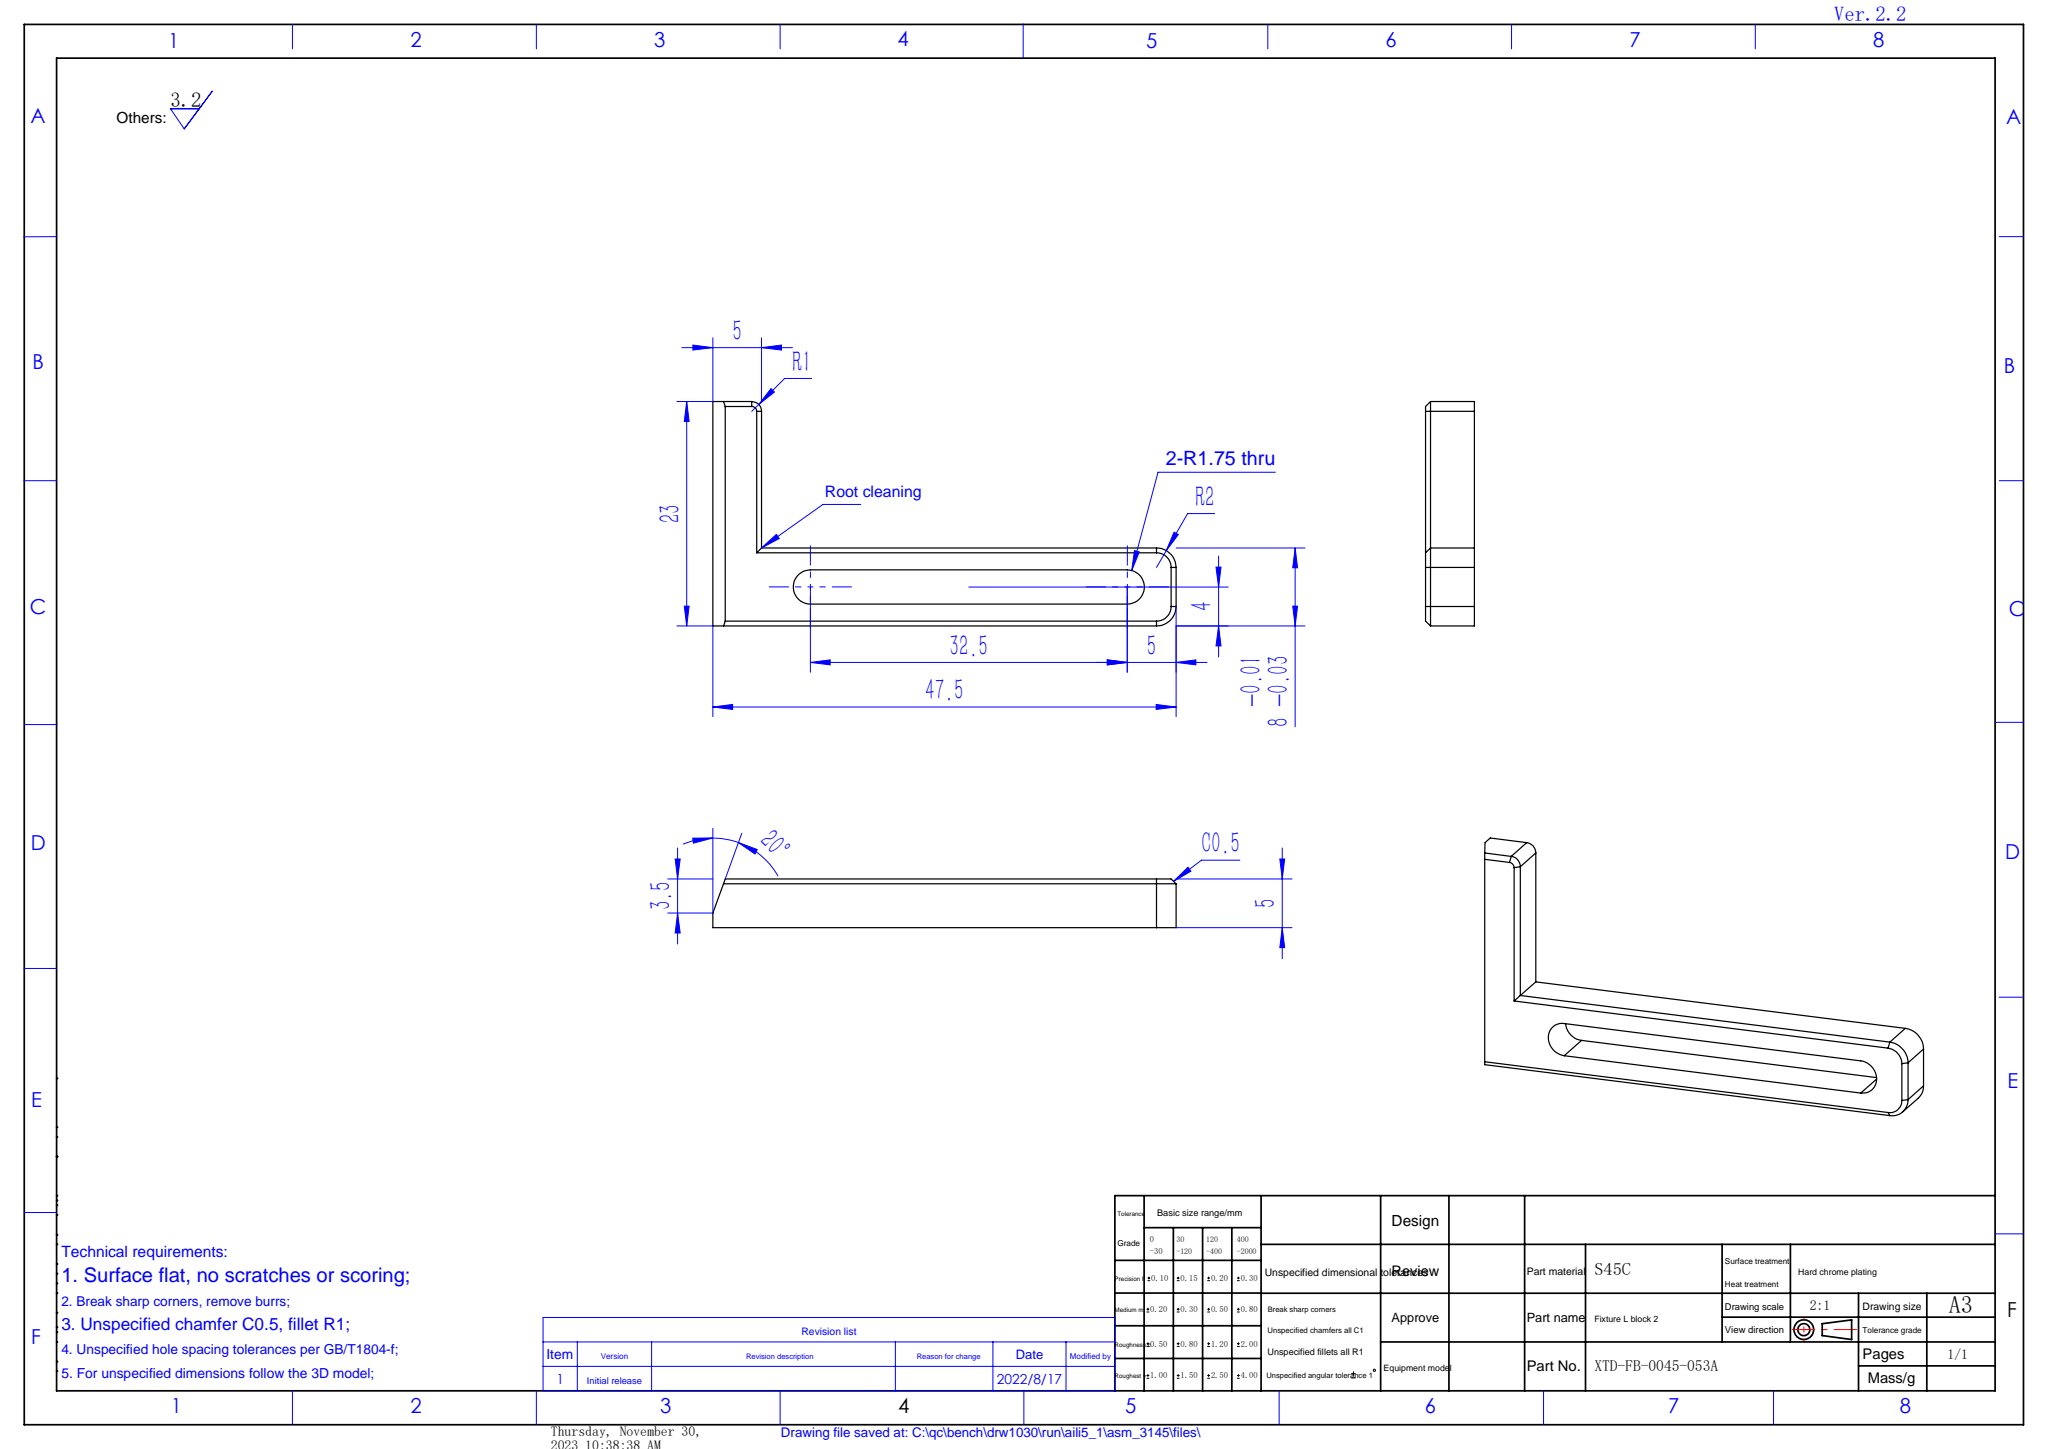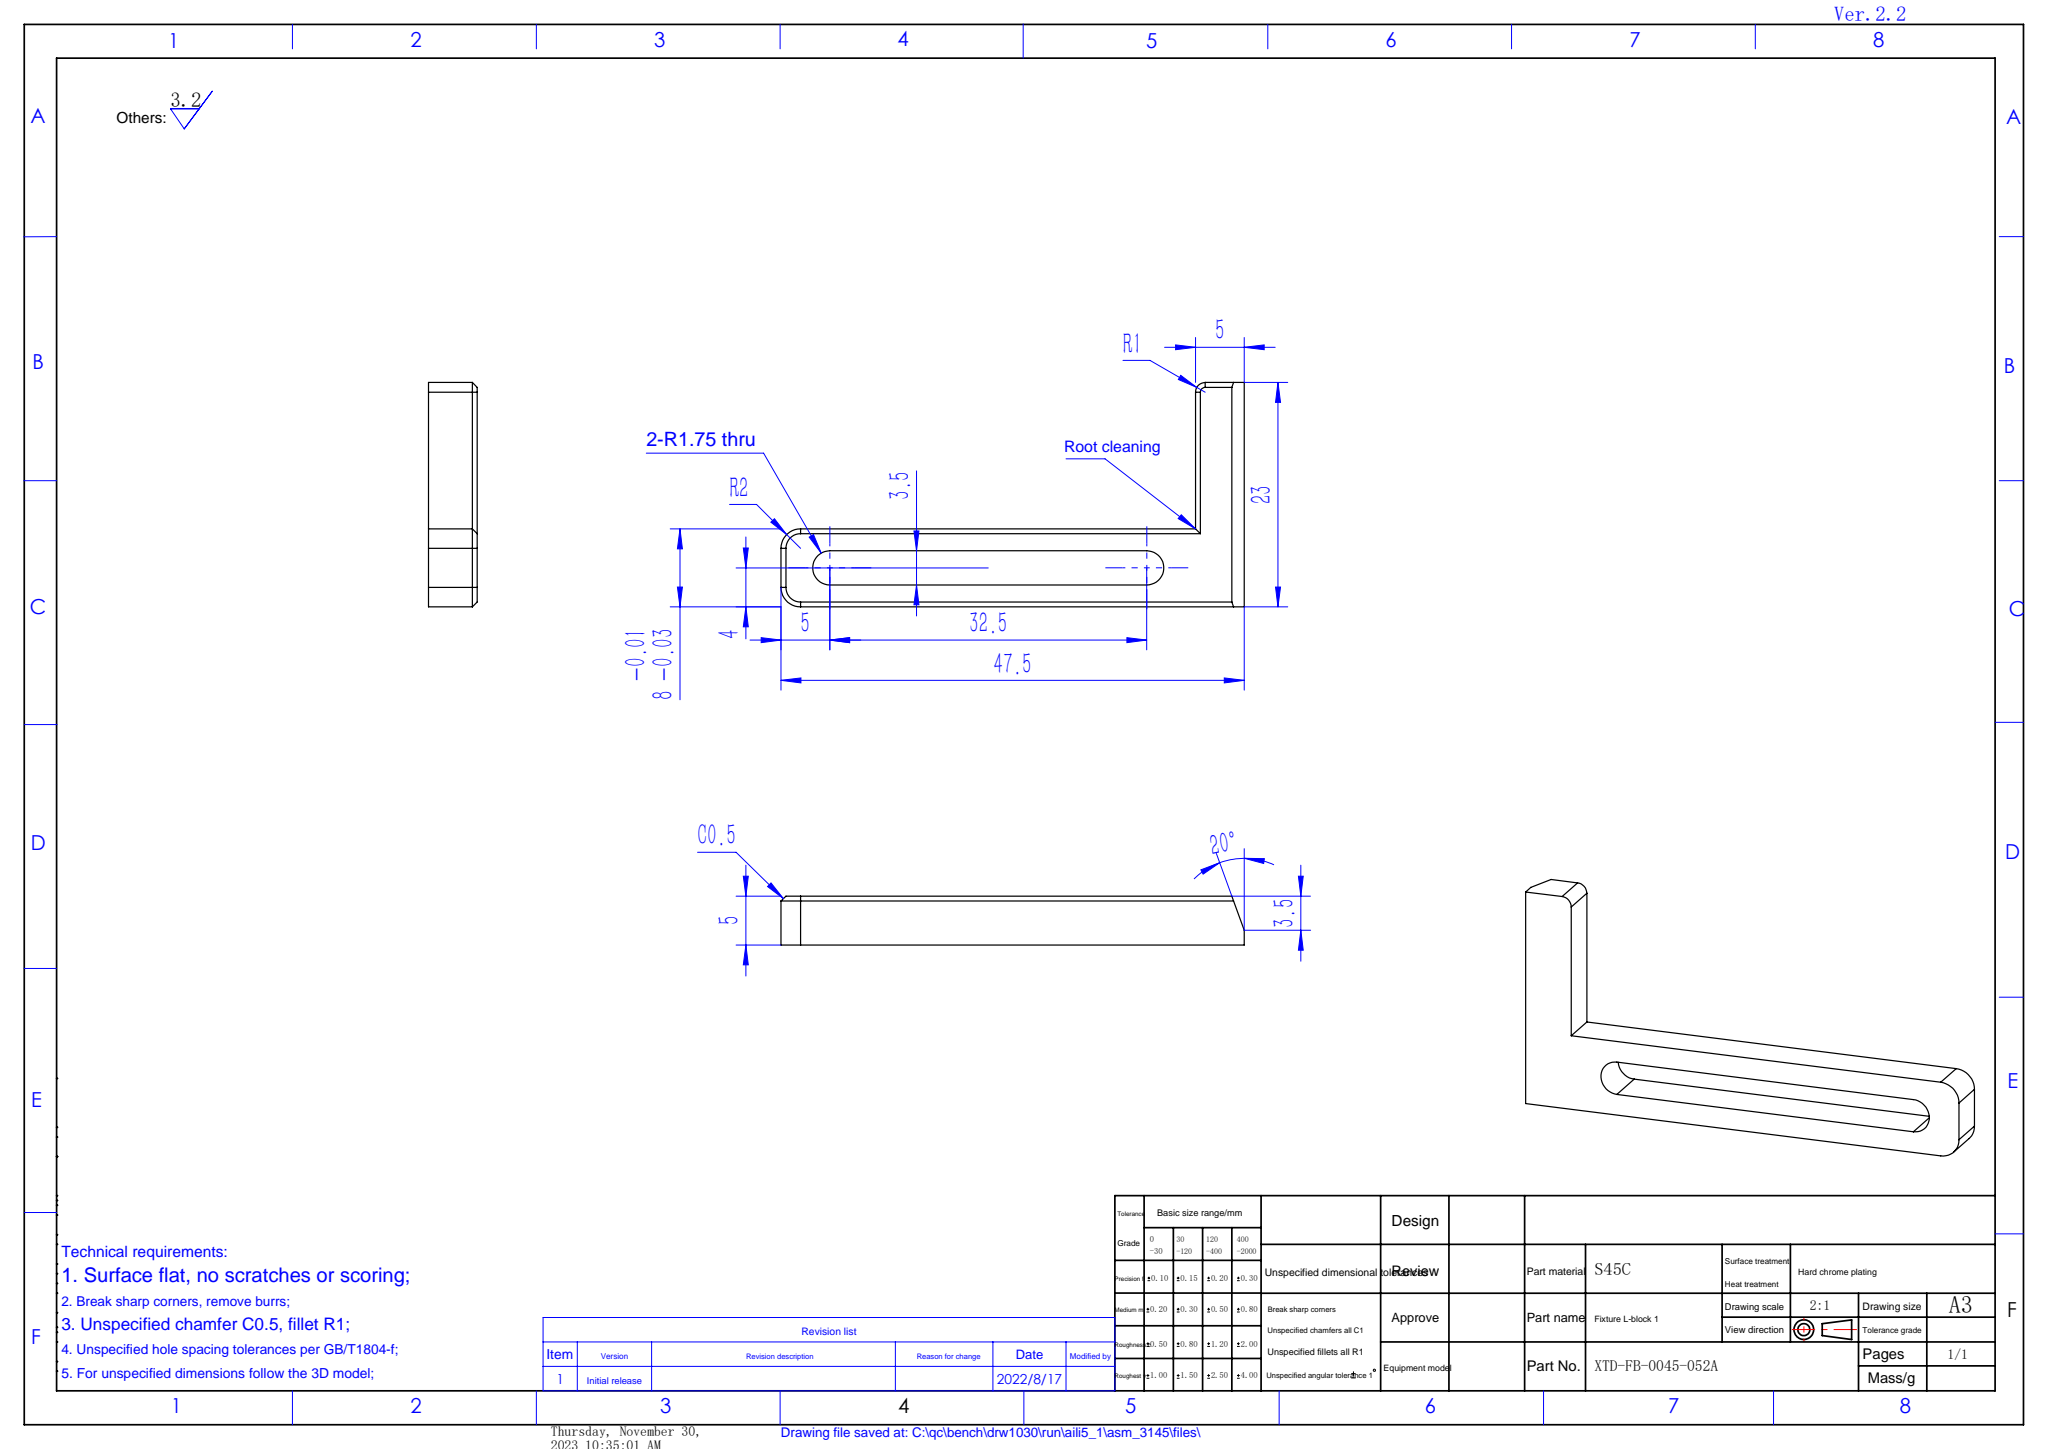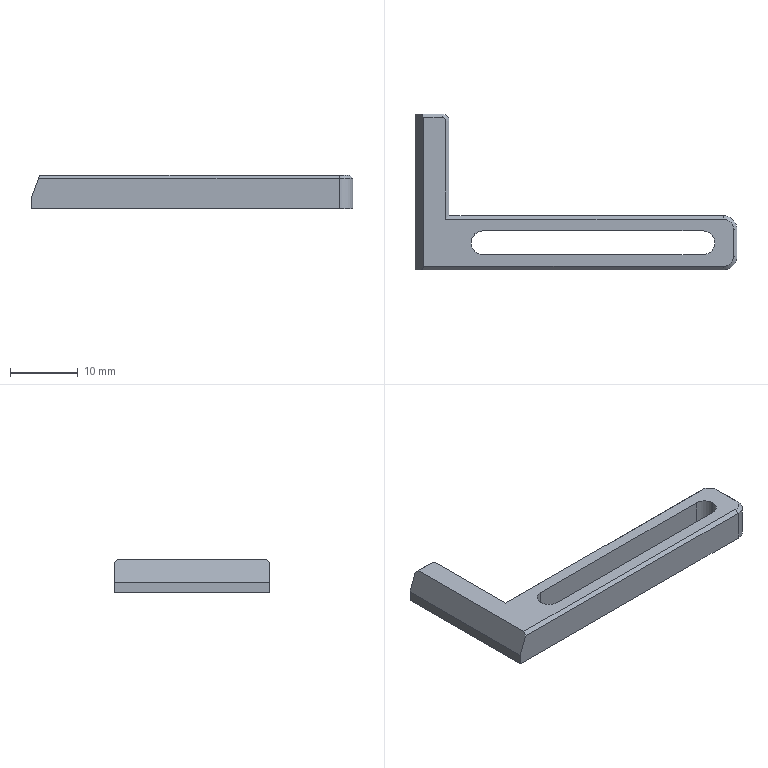Part | SolidWorks | features Fillet 2, Chamfer 1, Extrusion 1, HoleWzd 1, ICE 1 | 1 solid | 25 faces | box 47.5 x 23 x 5 mm | volume 1583 mm3 | plane 16 | cylinder 6 | cone 3 | commonest cylinder face diameters 3.5 x3 4 x2 2 x1
STEP:
#1=CARTESIAN_POINT('',(44.25,4.,0.));
#2=VERTEX_POINT('',#1);
#3=CARTESIAN_POINT('',(42.5,5.75,0.));
#4=VERTEX_POINT('',#3);
#5=CARTESIAN_POINT('',(42.5,4.,0.));
#6=DIRECTION('',(0.,0.,1.));
#7=DIRECTION('',(1.,0.,0.));
#8=AXIS2_PLACEMENT_3D('',#5,#6,#7);
#9=CIRCLE('',#8,1.75);
#10=EDGE_CURVE('',#2,#4,#9,.T.);
#11=ORIENTED_EDGE('',*,*,#10,.F.);
#12=CARTESIAN_POINT('',(44.25,4.,5.));
#13=VERTEX_POINT('',#12);
#14=CARTESIAN_POINT('',(44.25,4.,5.));
#15=DIRECTION('',(0.,0.,1.));
#16=VECTOR('',#15,1000.);
#17=LINE('',#14,#16);
#18=EDGE_CURVE('',#2,#13,#17,.T.);
#19=ORIENTED_EDGE('',*,*,#18,.T.);
#20=CARTESIAN_POINT('',(42.5,5.75,5.));
#21=VERTEX_POINT('',#20);
#22=CARTESIAN_POINT('',(42.5,4.,5.));
#23=DIRECTION('',(0.,0.,1.));
#24=DIRECTION('',(1.,0.,0.));
#25=AXIS2_PLACEMENT_3D('',#22,#23,#24);
#26=CIRCLE('',#25,1.75);
#27=EDGE_CURVE('',#13,#21,#26,.T.);
#28=ORIENTED_EDGE('',*,*,#27,.T.);
#29=CARTESIAN_POINT('',(42.5,5.75,5.));
#30=DIRECTION('',(0.,0.,1.));
#31=VECTOR('',#30,1000.);
#32=LINE('',#29,#31);
#33=EDGE_CURVE('',#4,#21,#32,.T.);
#34=ORIENTED_EDGE('',*,*,#33,.F.);
#35=EDGE_LOOP('',(#11,#19,#28,#34));
#36=FACE_OUTER_BOUND('',#35,.T.);
#37=CARTESIAN_POINT('',(42.5,4.,5.));
#38=DIRECTION('',(0.,0.,1.));
#39=DIRECTION('',(1.,0.,0.));
#40=AXIS2_PLACEMENT_3D('',#37,#38,#39);
#41=CYLINDRICAL_SURFACE('',#40,1.75);
#42=ADVANCED_FACE('',(#36),#41,.F.);
#43=CARTESIAN_POINT('',(4.5,22.,5.));
#44=VERTEX_POINT('',#43);
#45=CARTESIAN_POINT('',(4.,22.5,5.));
#46=VERTEX_POINT('',#45);
#47=CARTESIAN_POINT('',(4.,22.,5.));
#48=DIRECTION('',(0.,0.,1.));
#49=DIRECTION('',(-1.,0.,0.));
#50=AXIS2_PLACEMENT_3D('',#47,#48,#49);
#51=CIRCLE('',#50,0.5);
#52=EDGE_CURVE('',#44,#46,#51,.T.);
#53=ORIENTED_EDGE('',*,*,#52,.T.);
#54=CARTESIAN_POINT('',(1.274,22.5,5.));
#55=VERTEX_POINT('',#54);
#56=CARTESIAN_POINT('',(0.,22.5,5.));
#57=DIRECTION('',(-1.,0.,0.));
#58=VECTOR('',#57,1000.);
#59=LINE('',#56,#58);
#60=EDGE_CURVE('',#46,#55,#59,.T.);
#61=ORIENTED_EDGE('',*,*,#60,.T.);
#62=CARTESIAN_POINT('',(1.274,0.5,5.));
#63=VERTEX_POINT('',#62);
#64=CARTESIAN_POINT('',(1.274,23.,5.));
#65=DIRECTION('',(0.,-1.,0.));
#66=VECTOR('',#65,1000.);
#67=LINE('',#64,#66);
#68=EDGE_CURVE('',#55,#63,#67,.T.);
#69=ORIENTED_EDGE('',*,*,#68,.T.);
#70=CARTESIAN_POINT('',(45.5,0.5,5.));
#71=VERTEX_POINT('',#70);
#72=CARTESIAN_POINT('',(0.,0.5,5.));
#73=DIRECTION('',(1.,0.,0.));
#74=VECTOR('',#73,1000.);
#75=LINE('',#72,#74);
#76=EDGE_CURVE('',#63,#71,#75,.T.);
#77=ORIENTED_EDGE('',*,*,#76,.T.);
#78=CARTESIAN_POINT('',(47.,2.,5.));
#79=VERTEX_POINT('',#78);
#80=CARTESIAN_POINT('',(45.5,2.,5.));
#81=DIRECTION('',(0.,0.,1.));
#82=DIRECTION('',(-1.,0.,0.));
#83=AXIS2_PLACEMENT_3D('',#80,#81,#82);
#84=CIRCLE('',#83,1.5);
#85=EDGE_CURVE('',#71,#79,#84,.T.);
#86=ORIENTED_EDGE('',*,*,#85,.T.);
#87=CARTESIAN_POINT('',(47.,6.,5.));
#88=VERTEX_POINT('',#87);
#89=CARTESIAN_POINT('',(47.,0.,5.));
#90=DIRECTION('',(0.,1.,0.));
#91=VECTOR('',#90,1000.);
#92=LINE('',#89,#91);
#93=EDGE_CURVE('',#79,#88,#92,.T.);
#94=ORIENTED_EDGE('',*,*,#93,.T.);
#95=CARTESIAN_POINT('',(45.5,7.5,5.));
#96=VERTEX_POINT('',#95);
#97=CARTESIAN_POINT('',(45.5,6.,5.));
#98=DIRECTION('',(0.,0.,1.));
#99=DIRECTION('',(-1.,0.,0.));
#100=AXIS2_PLACEMENT_3D('',#97,#98,#99);
#101=CIRCLE('',#100,1.5);
#102=EDGE_CURVE('',#88,#96,#101,.T.);
#103=ORIENTED_EDGE('',*,*,#102,.T.);
#104=CARTESIAN_POINT('',(4.5,7.5,5.));
#105=VERTEX_POINT('',#104);
#106=CARTESIAN_POINT('',(0.,7.5,5.));
#107=DIRECTION('',(-1.,0.,0.));
#108=VECTOR('',#107,1000.);
#109=LINE('',#106,#108);
#110=EDGE_CURVE('',#96,#105,#109,.T.);
#111=ORIENTED_EDGE('',*,*,#110,.T.);
#112=CARTESIAN_POINT('',(4.5,0.,5.));
#113=DIRECTION('',(0.,1.,0.));
#114=VECTOR('',#113,1000.);
#115=LINE('',#112,#114);
#116=EDGE_CURVE('',#105,#44,#115,.T.);
#117=ORIENTED_EDGE('',*,*,#116,.T.);
#118=EDGE_LOOP('',(#53,#61,#69,#77,#86,#94,#103,#111,#117));
#119=FACE_OUTER_BOUND('',#118,.T.);
#120=CARTESIAN_POINT('',(10.,2.25,5.));
#121=VERTEX_POINT('',#120);
#122=CARTESIAN_POINT('',(42.5,2.25,5.));
#123=VERTEX_POINT('',#122);
#124=CARTESIAN_POINT('',(10.,2.25,5.));
#125=DIRECTION('',(1.,0.,0.));
#126=VECTOR('',#125,1000.);
#127=LINE('',#124,#126);
#128=EDGE_CURVE('',#121,#123,#127,.T.);
#129=ORIENTED_EDGE('',*,*,#128,.F.);
#130=CARTESIAN_POINT('',(10.,5.75,5.));
#131=VERTEX_POINT('',#130);
#132=CARTESIAN_POINT('',(10.,4.,5.));
#133=DIRECTION('',(0.,0.,1.));
#134=DIRECTION('',(1.,0.,0.));
#135=AXIS2_PLACEMENT_3D('',#132,#133,#134);
#136=CIRCLE('',#135,1.75);
#137=EDGE_CURVE('',#131,#121,#136,.T.);
#138=ORIENTED_EDGE('',*,*,#137,.F.);
#139=CARTESIAN_POINT('',(10.,5.75,5.));
#140=DIRECTION('',(1.,0.,0.));
#141=VECTOR('',#140,1000.);
#142=LINE('',#139,#141);
#143=EDGE_CURVE('',#131,#21,#142,.T.);
#144=ORIENTED_EDGE('',*,*,#143,.T.);
#145=ORIENTED_EDGE('',*,*,#27,.F.);
#146=CARTESIAN_POINT('',(42.5,4.,5.));
#147=DIRECTION('',(0.,0.,1.));
#148=DIRECTION('',(1.,0.,0.));
#149=AXIS2_PLACEMENT_3D('',#146,#147,#148);
#150=CIRCLE('',#149,1.75);
#151=EDGE_CURVE('',#123,#13,#150,.T.);
#152=ORIENTED_EDGE('',*,*,#151,.F.);
#153=EDGE_LOOP('',(#129,#138,#144,#145,#152));
#154=FACE_BOUND('',#153,.T.);
#155=CARTESIAN_POINT('',(0.,0.,5.));
#156=DIRECTION('',(0.,0.,-1.));
#157=DIRECTION('',(-1.,0.,0.));
#158=AXIS2_PLACEMENT_3D('',#155,#156,#157);
#159=PLANE('',#158);
#160=ADVANCED_FACE('',(#119,#154),#159,.F.);
#161=CARTESIAN_POINT('',(47.5,2.,0.));
#162=VERTEX_POINT('',#161);
#163=CARTESIAN_POINT('',(47.5,6.,0.));
#164=VERTEX_POINT('',#163);
#165=CARTESIAN_POINT('',(47.5,8.,0.));
#166=DIRECTION('',(0.,1.,0.));
#167=VECTOR('',#166,1000.);
#168=LINE('',#165,#167);
#169=EDGE_CURVE('',#162,#164,#168,.T.);
#170=ORIENTED_EDGE('',*,*,#169,.F.);
#171=CARTESIAN_POINT('',(45.5,0.,0.));
#172=VERTEX_POINT('',#171);
#173=CARTESIAN_POINT('',(45.5,2.,0.));
#174=DIRECTION('',(0.,0.,-1.));
#175=DIRECTION('',(-1.,0.,0.));
#176=AXIS2_PLACEMENT_3D('',#173,#174,#175);
#177=CIRCLE('',#176,2.);
#178=EDGE_CURVE('',#162,#172,#177,.T.);
#179=ORIENTED_EDGE('',*,*,#178,.T.);
#180=CARTESIAN_POINT('',(0.,0.,0.));
#181=VERTEX_POINT('',#180);
#182=CARTESIAN_POINT('',(47.5,0.,0.));
#183=DIRECTION('',(1.,0.,0.));
#184=VECTOR('',#183,1000.);
#185=LINE('',#182,#184);
#186=EDGE_CURVE('',#181,#172,#185,.T.);
#187=ORIENTED_EDGE('',*,*,#186,.F.);
#188=CARTESIAN_POINT('',(0.,23.,0.));
#189=VERTEX_POINT('',#188);
#190=CARTESIAN_POINT('',(0.,0.,0.));
#191=DIRECTION('',(0.,-1.,0.));
#192=VECTOR('',#191,1000.);
#193=LINE('',#190,#192);
#194=EDGE_CURVE('',#189,#181,#193,.T.);
#195=ORIENTED_EDGE('',*,*,#194,.F.);
#196=CARTESIAN_POINT('',(4.,23.,0.));
#197=VERTEX_POINT('',#196);
#198=CARTESIAN_POINT('',(0.,23.,0.));
#199=DIRECTION('',(-1.,0.,0.));
#200=VECTOR('',#199,1000.);
#201=LINE('',#198,#200);
#202=EDGE_CURVE('',#197,#189,#201,.T.);
#203=ORIENTED_EDGE('',*,*,#202,.F.);
#204=CARTESIAN_POINT('',(5.,22.,0.));
#205=VERTEX_POINT('',#204);
#206=CARTESIAN_POINT('',(4.,22.,0.));
#207=DIRECTION('',(0.,0.,-1.));
#208=DIRECTION('',(-1.,0.,0.));
#209=AXIS2_PLACEMENT_3D('',#206,#207,#208);
#210=CIRCLE('',#209,1.);
#211=EDGE_CURVE('',#197,#205,#210,.T.);
#212=ORIENTED_EDGE('',*,*,#211,.T.);
#213=CARTESIAN_POINT('',(5.,8.,0.));
#214=VERTEX_POINT('',#213);
#215=CARTESIAN_POINT('',(5.,23.,0.));
#216=DIRECTION('',(0.,1.,0.));
#217=VECTOR('',#216,1000.);
#218=LINE('',#215,#217);
#219=EDGE_CURVE('',#214,#205,#218,.T.);
#220=ORIENTED_EDGE('',*,*,#219,.F.);
#221=CARTESIAN_POINT('',(45.5,8.,0.));
#222=VERTEX_POINT('',#221);
#223=CARTESIAN_POINT('',(5.,8.,0.));
#224=DIRECTION('',(-1.,0.,0.));
#225=VECTOR('',#224,1000.);
#226=LINE('',#223,#225);
#227=EDGE_CURVE('',#222,#214,#226,.T.);
#228=ORIENTED_EDGE('',*,*,#227,.F.);
#229=CARTESIAN_POINT('',(45.5,6.,0.));
#230=DIRECTION('',(0.,0.,-1.));
#231=DIRECTION('',(-1.,0.,0.));
#232=AXIS2_PLACEMENT_3D('',#229,#230,#231);
#233=CIRCLE('',#232,2.);
#234=EDGE_CURVE('',#222,#164,#233,.T.);
#235=ORIENTED_EDGE('',*,*,#234,.T.);
#236=EDGE_LOOP('',(#170,#179,#187,#195,#203,#212,#220,#228,#235));
#237=FACE_OUTER_BOUND('',#236,.T.);
#238=CARTESIAN_POINT('',(10.,2.25,0.));
#239=VERTEX_POINT('',#238);
#240=CARTESIAN_POINT('',(42.5,2.25,0.));
#241=VERTEX_POINT('',#240);
#242=CARTESIAN_POINT('',(10.,2.25,0.));
#243=DIRECTION('',(1.,0.,0.));
#244=VECTOR('',#243,1000.);
#245=LINE('',#242,#244);
#246=EDGE_CURVE('',#239,#241,#245,.T.);
#247=ORIENTED_EDGE('',*,*,#246,.T.);
#248=CARTESIAN_POINT('',(42.5,4.,0.));
#249=DIRECTION('',(0.,0.,1.));
#250=DIRECTION('',(1.,0.,0.));
#251=AXIS2_PLACEMENT_3D('',#248,#249,#250);
#252=CIRCLE('',#251,1.75);
#253=EDGE_CURVE('',#241,#2,#252,.T.);
#254=ORIENTED_EDGE('',*,*,#253,.T.);
#255=ORIENTED_EDGE('',*,*,#10,.T.);
#256=CARTESIAN_POINT('',(10.,5.75,0.));
#257=VERTEX_POINT('',#256);
#258=CARTESIAN_POINT('',(10.,5.75,0.));
#259=DIRECTION('',(1.,0.,0.));
#260=VECTOR('',#259,1000.);
#261=LINE('',#258,#260);
#262=EDGE_CURVE('',#257,#4,#261,.T.);
#263=ORIENTED_EDGE('',*,*,#262,.F.);
#264=CARTESIAN_POINT('',(10.,4.,0.));
#265=DIRECTION('',(0.,0.,1.));
#266=DIRECTION('',(1.,0.,0.));
#267=AXIS2_PLACEMENT_3D('',#264,#265,#266);
#268=CIRCLE('',#267,1.75);
#269=EDGE_CURVE('',#257,#239,#268,.T.);
#270=ORIENTED_EDGE('',*,*,#269,.T.);
#271=EDGE_LOOP('',(#247,#254,#255,#263,#270));
#272=FACE_BOUND('',#271,.T.);
#273=CARTESIAN_POINT('',(0.,0.,0.));
#274=DIRECTION('',(0.,0.,-1.));
#275=DIRECTION('',(-1.,0.,0.));
#276=AXIS2_PLACEMENT_3D('',#273,#274,#275);
#277=PLANE('',#276);
#278=ADVANCED_FACE('',(#237,#272),#277,.T.);
#279=CARTESIAN_POINT('',(45.5,0.,4.5));
#280=VERTEX_POINT('',#279);
#281=CARTESIAN_POINT('',(45.5,0.,5.));
#282=DIRECTION('',(0.,0.,1.));
#283=VECTOR('',#282,1000.);
#284=LINE('',#281,#283);
#285=EDGE_CURVE('',#172,#280,#284,.T.);
#286=ORIENTED_EDGE('',*,*,#285,.T.);
#287=CARTESIAN_POINT('',(1.092,0.,4.5));
#288=VERTEX_POINT('',#287);
#289=CARTESIAN_POINT('',(47.5,0.,4.5));
#290=DIRECTION('',(-1.,0.,0.));
#291=VECTOR('',#290,1000.);
#292=LINE('',#289,#291);
#293=EDGE_CURVE('',#280,#288,#292,.T.);
#294=ORIENTED_EDGE('',*,*,#293,.T.);
#295=CARTESIAN_POINT('',(0.,0.,1.5));
#296=VERTEX_POINT('',#295);
#297=CARTESIAN_POINT('',(1.274,0.,5.));
#298=DIRECTION('',(0.342,0.,0.9397));
#299=VECTOR('',#298,1000.);
#300=LINE('',#297,#299);
#301=EDGE_CURVE('',#296,#288,#300,.T.);
#302=ORIENTED_EDGE('',*,*,#301,.F.);
#303=CARTESIAN_POINT('',(0.,0.,5.));
#304=DIRECTION('',(0.,0.,-1.));
#305=VECTOR('',#304,1000.);
#306=LINE('',#303,#305);
#307=EDGE_CURVE('',#296,#181,#306,.T.);
#308=ORIENTED_EDGE('',*,*,#307,.T.);
#309=ORIENTED_EDGE('',*,*,#186,.T.);
#310=EDGE_LOOP('',(#286,#294,#302,#308,#309));
#311=FACE_OUTER_BOUND('',#310,.T.);
#312=CARTESIAN_POINT('',(47.5,0.,5.));
#313=DIRECTION('',(0.,1.,0.));
#314=DIRECTION('',(-1.,0.,0.));
#315=AXIS2_PLACEMENT_3D('',#312,#313,#314);
#316=PLANE('',#315);
#317=ADVANCED_FACE('',(#311),#316,.F.);
#318=CARTESIAN_POINT('',(47.5,6.,4.5));
#319=VERTEX_POINT('',#318);
#320=CARTESIAN_POINT('',(47.5,6.,5.));
#321=DIRECTION('',(0.,0.,1.));
#322=VECTOR('',#321,1000.);
#323=LINE('',#320,#322);
#324=EDGE_CURVE('',#164,#319,#323,.T.);
#325=ORIENTED_EDGE('',*,*,#324,.T.);
#326=CARTESIAN_POINT('',(47.5,2.,4.5));
#327=VERTEX_POINT('',#326);
#328=CARTESIAN_POINT('',(47.5,8.,4.5));
#329=DIRECTION('',(0.,-1.,0.));
#330=VECTOR('',#329,1000.);
#331=LINE('',#328,#330);
#332=EDGE_CURVE('',#319,#327,#331,.T.);
#333=ORIENTED_EDGE('',*,*,#332,.T.);
#334=CARTESIAN_POINT('',(47.5,2.,5.));
#335=DIRECTION('',(0.,0.,-1.));
#336=VECTOR('',#335,1000.);
#337=LINE('',#334,#336);
#338=EDGE_CURVE('',#327,#162,#337,.T.);
#339=ORIENTED_EDGE('',*,*,#338,.T.);
#340=ORIENTED_EDGE('',*,*,#169,.T.);
#341=EDGE_LOOP('',(#325,#333,#339,#340));
#342=FACE_OUTER_BOUND('',#341,.T.);
#343=CARTESIAN_POINT('',(47.5,8.,5.));
#344=DIRECTION('',(-1.,0.,0.));
#345=DIRECTION('',(0.,0.,1.));
#346=AXIS2_PLACEMENT_3D('',#343,#344,#345);
#347=PLANE('',#346);
#348=ADVANCED_FACE('',(#342),#347,.F.);
#349=CARTESIAN_POINT('',(5.,8.,4.5));
#350=VERTEX_POINT('',#349);
#351=CARTESIAN_POINT('',(5.,8.,5.));
#352=DIRECTION('',(0.,0.,-1.));
#353=VECTOR('',#352,1000.);
#354=LINE('',#351,#353);
#355=EDGE_CURVE('',#350,#214,#354,.T.);
#356=ORIENTED_EDGE('',*,*,#355,.F.);
#357=CARTESIAN_POINT('',(45.5,8.,4.5));
#358=VERTEX_POINT('',#357);
#359=CARTESIAN_POINT('',(5.,8.,4.5));
#360=DIRECTION('',(1.,0.,0.));
#361=VECTOR('',#360,1000.);
#362=LINE('',#359,#361);
#363=EDGE_CURVE('',#350,#358,#362,.T.);
#364=ORIENTED_EDGE('',*,*,#363,.T.);
#365=CARTESIAN_POINT('',(45.5,8.,5.));
#366=DIRECTION('',(0.,0.,-1.));
#367=VECTOR('',#366,1000.);
#368=LINE('',#365,#367);
#369=EDGE_CURVE('',#358,#222,#368,.T.);
#370=ORIENTED_EDGE('',*,*,#369,.T.);
#371=ORIENTED_EDGE('',*,*,#227,.T.);
#372=EDGE_LOOP('',(#356,#364,#370,#371));
#373=FACE_OUTER_BOUND('',#372,.T.);
#374=CARTESIAN_POINT('',(5.,8.,5.));
#375=DIRECTION('',(0.,-1.,0.));
#376=DIRECTION('',(1.,0.,0.));
#377=AXIS2_PLACEMENT_3D('',#374,#375,#376);
#378=PLANE('',#377);
#379=ADVANCED_FACE('',(#373),#378,.F.);
#380=CARTESIAN_POINT('',(5.,22.,4.5));
#381=VERTEX_POINT('',#380);
#382=CARTESIAN_POINT('',(5.,22.,5.));
#383=DIRECTION('',(0.,0.,1.));
#384=VECTOR('',#383,1000.);
#385=LINE('',#382,#384);
#386=EDGE_CURVE('',#205,#381,#385,.T.);
#387=ORIENTED_EDGE('',*,*,#386,.T.);
#388=CARTESIAN_POINT('',(5.,23.,4.5));
#389=DIRECTION('',(0.,-1.,0.));
#390=VECTOR('',#389,1000.);
#391=LINE('',#388,#390);
#392=EDGE_CURVE('',#381,#350,#391,.T.);
#393=ORIENTED_EDGE('',*,*,#392,.T.);
#394=ORIENTED_EDGE('',*,*,#355,.T.);
#395=ORIENTED_EDGE('',*,*,#219,.T.);
#396=EDGE_LOOP('',(#387,#393,#394,#395));
#397=FACE_OUTER_BOUND('',#396,.T.);
#398=CARTESIAN_POINT('',(5.,23.,5.));
#399=DIRECTION('',(-1.,0.,0.));
#400=DIRECTION('',(0.,-1.,0.));
#401=AXIS2_PLACEMENT_3D('',#398,#399,#400);
#402=PLANE('',#401);
#403=ADVANCED_FACE('',(#397),#402,.F.);
#404=CARTESIAN_POINT('',(0.,23.,1.5));
#405=VERTEX_POINT('',#404);
#406=CARTESIAN_POINT('',(1.092,23.,4.5));
#407=VERTEX_POINT('',#406);
#408=CARTESIAN_POINT('',(1.274,23.,5.));
#409=DIRECTION('',(0.342,0.,0.9397));
#410=VECTOR('',#409,1000.);
#411=LINE('',#408,#410);
#412=EDGE_CURVE('',#405,#407,#411,.T.);
#413=ORIENTED_EDGE('',*,*,#412,.T.);
#414=CARTESIAN_POINT('',(4.,23.,4.5));
#415=VERTEX_POINT('',#414);
#416=CARTESIAN_POINT('',(0.,23.,4.5));
#417=DIRECTION('',(1.,0.,0.));
#418=VECTOR('',#417,1000.);
#419=LINE('',#416,#418);
#420=EDGE_CURVE('',#407,#415,#419,.T.);
#421=ORIENTED_EDGE('',*,*,#420,.T.);
#422=CARTESIAN_POINT('',(4.,23.,5.));
#423=DIRECTION('',(0.,0.,-1.));
#424=VECTOR('',#423,1000.);
#425=LINE('',#422,#424);
#426=EDGE_CURVE('',#415,#197,#425,.T.);
#427=ORIENTED_EDGE('',*,*,#426,.T.);
#428=ORIENTED_EDGE('',*,*,#202,.T.);
#429=CARTESIAN_POINT('',(0.,23.,5.));
#430=DIRECTION('',(0.,0.,-1.));
#431=VECTOR('',#430,1000.);
#432=LINE('',#429,#431);
#433=EDGE_CURVE('',#405,#189,#432,.T.);
#434=ORIENTED_EDGE('',*,*,#433,.F.);
#435=EDGE_LOOP('',(#413,#421,#427,#428,#434));
#436=FACE_OUTER_BOUND('',#435,.T.);
#437=CARTESIAN_POINT('',(0.,23.,5.));
#438=DIRECTION('',(0.,-1.,0.));
#439=DIRECTION('',(0.,0.,-1.));
#440=AXIS2_PLACEMENT_3D('',#437,#438,#439);
#441=PLANE('',#440);
#442=ADVANCED_FACE('',(#436),#441,.F.);
#443=ORIENTED_EDGE('',*,*,#307,.F.);
#444=CARTESIAN_POINT('',(0.,23.,1.5));
#445=DIRECTION('',(0.,-1.,0.));
#446=VECTOR('',#445,1000.);
#447=LINE('',#444,#446);
#448=EDGE_CURVE('',#405,#296,#447,.T.);
#449=ORIENTED_EDGE('',*,*,#448,.F.);
#450=ORIENTED_EDGE('',*,*,#433,.T.);
#451=ORIENTED_EDGE('',*,*,#194,.T.);
#452=EDGE_LOOP('',(#443,#449,#450,#451));
#453=FACE_OUTER_BOUND('',#452,.T.);
#454=CARTESIAN_POINT('',(0.,0.,5.));
#455=DIRECTION('',(1.,0.,0.));
#456=DIRECTION('',(0.,0.,-1.));
#457=AXIS2_PLACEMENT_3D('',#454,#455,#456);
#458=PLANE('',#457);
#459=ADVANCED_FACE('',(#453),#458,.F.);
#460=ORIENTED_EDGE('',*,*,#18,.F.);
#461=ORIENTED_EDGE('',*,*,#253,.F.);
#462=CARTESIAN_POINT('',(42.5,2.25,5.));
#463=DIRECTION('',(0.,0.,-1.));
#464=VECTOR('',#463,1000.);
#465=LINE('',#462,#464);
#466=EDGE_CURVE('',#123,#241,#465,.T.);
#467=ORIENTED_EDGE('',*,*,#466,.F.);
#468=ORIENTED_EDGE('',*,*,#151,.T.);
#469=EDGE_LOOP('',(#460,#461,#467,#468));
#470=FACE_OUTER_BOUND('',#469,.T.);
#471=CARTESIAN_POINT('',(42.5,4.,5.));
#472=DIRECTION('',(0.,0.,1.));
#473=DIRECTION('',(1.,0.,0.));
#474=AXIS2_PLACEMENT_3D('',#471,#472,#473);
#475=CYLINDRICAL_SURFACE('',#474,1.75);
#476=ADVANCED_FACE('',(#470),#475,.F.);
#477=ORIENTED_EDGE('',*,*,#137,.T.);
#478=CARTESIAN_POINT('',(10.,2.25,5.));
#479=DIRECTION('',(0.,0.,1.));
#480=VECTOR('',#479,1000.);
#481=LINE('',#478,#480);
#482=EDGE_CURVE('',#239,#121,#481,.T.);
#483=ORIENTED_EDGE('',*,*,#482,.F.);
#484=ORIENTED_EDGE('',*,*,#269,.F.);
#485=CARTESIAN_POINT('',(10.,5.75,5.));
#486=DIRECTION('',(0.,0.,-1.));
#487=VECTOR('',#486,1000.);
#488=LINE('',#485,#487);
#489=EDGE_CURVE('',#131,#257,#488,.T.);
#490=ORIENTED_EDGE('',*,*,#489,.F.);
#491=EDGE_LOOP('',(#477,#483,#484,#490));
#492=FACE_OUTER_BOUND('',#491,.T.);
#493=CARTESIAN_POINT('',(10.,4.,5.));
#494=DIRECTION('',(0.,0.,1.));
#495=DIRECTION('',(1.,0.,0.));
#496=AXIS2_PLACEMENT_3D('',#493,#494,#495);
#497=CYLINDRICAL_SURFACE('',#496,1.75);
#498=ADVANCED_FACE('',(#492),#497,.F.);
#499=ORIENTED_EDGE('',*,*,#33,.T.);
#500=ORIENTED_EDGE('',*,*,#143,.F.);
#501=ORIENTED_EDGE('',*,*,#489,.T.);
#502=ORIENTED_EDGE('',*,*,#262,.T.);
#503=EDGE_LOOP('',(#499,#500,#501,#502));
#504=FACE_OUTER_BOUND('',#503,.T.);
#505=CARTESIAN_POINT('',(10.,5.75,5.));
#506=DIRECTION('',(0.,1.,0.));
#507=DIRECTION('',(-1.,0.,0.));
#508=AXIS2_PLACEMENT_3D('',#505,#506,#507);
#509=PLANE('',#508);
#510=ADVANCED_FACE('',(#504),#509,.F.);
#511=ORIENTED_EDGE('',*,*,#466,.T.);
#512=ORIENTED_EDGE('',*,*,#246,.F.);
#513=ORIENTED_EDGE('',*,*,#482,.T.);
#514=ORIENTED_EDGE('',*,*,#128,.T.);
#515=EDGE_LOOP('',(#511,#512,#513,#514));
#516=FACE_OUTER_BOUND('',#515,.T.);
#517=CARTESIAN_POINT('',(10.,2.25,5.));
#518=DIRECTION('',(0.,-1.,0.));
#519=DIRECTION('',(1.,0.,0.));
#520=AXIS2_PLACEMENT_3D('',#517,#518,#519);
#521=PLANE('',#520);
#522=ADVANCED_FACE('',(#516),#521,.F.);
#523=ORIENTED_EDGE('',*,*,#68,.F.);
#524=CARTESIAN_POINT('',(1.195,22.717,4.783));
#525=DIRECTION('',(-0.2492,0.6848,-0.6848));
#526=VECTOR('',#525,1000.);
#527=LINE('',#524,#526);
#528=EDGE_CURVE('',#55,#407,#527,.T.);
#529=ORIENTED_EDGE('',*,*,#528,.T.);
#530=ORIENTED_EDGE('',*,*,#412,.F.);
#531=ORIENTED_EDGE('',*,*,#448,.T.);
#532=ORIENTED_EDGE('',*,*,#301,.T.);
#533=CARTESIAN_POINT('',(1.195,0.2826,4.783));
#534=DIRECTION('',(0.2492,0.6848,0.6848));
#535=VECTOR('',#534,1000.);
#536=LINE('',#533,#535);
#537=EDGE_CURVE('',#288,#63,#536,.T.);
#538=ORIENTED_EDGE('',*,*,#537,.T.);
#539=EDGE_LOOP('',(#523,#529,#530,#531,#532,#538));
#540=FACE_OUTER_BOUND('',#539,.T.);
#541=CARTESIAN_POINT('',(1.274,23.,5.));
#542=DIRECTION('',(0.9397,0.,-0.342));
#543=DIRECTION('',(-0.342,0.,-0.9397));
#544=AXIS2_PLACEMENT_3D('',#541,#542,#543);
#545=PLANE('',#544);
#546=ADVANCED_FACE('',(#540),#545,.F.);
#547=ORIENTED_EDGE('',*,*,#426,.F.);
#548=CARTESIAN_POINT('',(4.,22.,4.5));
#549=DIRECTION('',(0.,0.,-1.));
#550=DIRECTION('',(-1.,0.,0.));
#551=AXIS2_PLACEMENT_3D('',#548,#549,#550);
#552=CIRCLE('',#551,1.);
#553=EDGE_CURVE('',#415,#381,#552,.T.);
#554=ORIENTED_EDGE('',*,*,#553,.T.);
#555=ORIENTED_EDGE('',*,*,#386,.F.);
#556=ORIENTED_EDGE('',*,*,#211,.F.);
#557=EDGE_LOOP('',(#547,#554,#555,#556));
#558=FACE_OUTER_BOUND('',#557,.T.);
#559=CARTESIAN_POINT('',(4.,22.,5.));
#560=DIRECTION('',(0.,0.,-1.));
#561=DIRECTION('',(-1.,0.,0.));
#562=AXIS2_PLACEMENT_3D('',#559,#560,#561);
#563=CYLINDRICAL_SURFACE('',#562,1.);
#564=ADVANCED_FACE('',(#558),#563,.T.);
#565=ORIENTED_EDGE('',*,*,#338,.F.);
#566=CARTESIAN_POINT('',(45.5,2.,4.5));
#567=DIRECTION('',(0.,0.,-1.));
#568=DIRECTION('',(-1.,0.,0.));
#569=AXIS2_PLACEMENT_3D('',#566,#567,#568);
#570=CIRCLE('',#569,2.);
#571=EDGE_CURVE('',#327,#280,#570,.T.);
#572=ORIENTED_EDGE('',*,*,#571,.T.);
#573=ORIENTED_EDGE('',*,*,#285,.F.);
#574=ORIENTED_EDGE('',*,*,#178,.F.);
#575=EDGE_LOOP('',(#565,#572,#573,#574));
#576=FACE_OUTER_BOUND('',#575,.T.);
#577=CARTESIAN_POINT('',(45.5,2.,5.));
#578=DIRECTION('',(0.,0.,-1.));
#579=DIRECTION('',(-1.,0.,0.));
#580=AXIS2_PLACEMENT_3D('',#577,#578,#579);
#581=CYLINDRICAL_SURFACE('',#580,2.);
#582=ADVANCED_FACE('',(#576),#581,.T.);
#583=ORIENTED_EDGE('',*,*,#369,.F.);
#584=CARTESIAN_POINT('',(45.5,6.,4.5));
#585=DIRECTION('',(0.,0.,-1.));
#586=DIRECTION('',(-1.,0.,0.));
#587=AXIS2_PLACEMENT_3D('',#584,#585,#586);
#588=CIRCLE('',#587,2.);
#589=EDGE_CURVE('',#358,#319,#588,.T.);
#590=ORIENTED_EDGE('',*,*,#589,.T.);
#591=ORIENTED_EDGE('',*,*,#324,.F.);
#592=ORIENTED_EDGE('',*,*,#234,.F.);
#593=EDGE_LOOP('',(#583,#590,#591,#592));
#594=FACE_OUTER_BOUND('',#593,.T.);
#595=CARTESIAN_POINT('',(45.5,6.,5.));
#596=DIRECTION('',(0.,0.,-1.));
#597=DIRECTION('',(-1.,0.,0.));
#598=AXIS2_PLACEMENT_3D('',#595,#596,#597);
#599=CYLINDRICAL_SURFACE('',#598,2.);
#600=ADVANCED_FACE('',(#594),#599,.T.);
#601=ORIENTED_EDGE('',*,*,#537,.F.);
#602=ORIENTED_EDGE('',*,*,#293,.F.);
#603=CARTESIAN_POINT('',(45.5,0.5,5.));
#604=DIRECTION('',(0.,-0.7071,-0.7071));
#605=VECTOR('',#604,1000.);
#606=LINE('',#603,#605);
#607=EDGE_CURVE('',#71,#280,#606,.T.);
#608=ORIENTED_EDGE('',*,*,#607,.F.);
#609=ORIENTED_EDGE('',*,*,#76,.F.);
#610=EDGE_LOOP('',(#601,#602,#608,#609));
#611=FACE_OUTER_BOUND('',#610,.T.);
#612=CARTESIAN_POINT('',(0.,0.5,5.));
#613=DIRECTION('',(0.,0.7071,-0.7071));
#614=DIRECTION('',(1.,0.,0.));
#615=AXIS2_PLACEMENT_3D('',#612,#613,#614);
#616=PLANE('',#615);
#617=ADVANCED_FACE('',(#611),#616,.F.);
#618=ORIENTED_EDGE('',*,*,#607,.T.);
#619=ORIENTED_EDGE('',*,*,#571,.F.);
#620=CARTESIAN_POINT('',(47.,2.,5.));
#621=DIRECTION('',(0.7071,0.,-0.7071));
#622=VECTOR('',#621,1000.);
#623=LINE('',#620,#622);
#624=EDGE_CURVE('',#79,#327,#623,.T.);
#625=ORIENTED_EDGE('',*,*,#624,.F.);
#626=ORIENTED_EDGE('',*,*,#85,.F.);
#627=EDGE_LOOP('',(#618,#619,#625,#626));
#628=FACE_OUTER_BOUND('',#627,.T.);
#629=CARTESIAN_POINT('',(45.5,2.,5.));
#630=DIRECTION('',(0.,0.,-1.));
#631=DIRECTION('',(-1.,0.,0.));
#632=AXIS2_PLACEMENT_3D('',#629,#630,#631);
#633=CONICAL_SURFACE('',#632,1.5,0.7854);
#634=ADVANCED_FACE('',(#628),#633,.T.);
#635=ORIENTED_EDGE('',*,*,#624,.T.);
#636=ORIENTED_EDGE('',*,*,#332,.F.);
#637=CARTESIAN_POINT('',(47.,6.,5.));
#638=DIRECTION('',(0.7071,0.,-0.7071));
#639=VECTOR('',#638,1000.);
#640=LINE('',#637,#639);
#641=EDGE_CURVE('',#88,#319,#640,.T.);
#642=ORIENTED_EDGE('',*,*,#641,.F.);
#643=ORIENTED_EDGE('',*,*,#93,.F.);
#644=EDGE_LOOP('',(#635,#636,#642,#643));
#645=FACE_OUTER_BOUND('',#644,.T.);
#646=CARTESIAN_POINT('',(47.,0.,5.));
#647=DIRECTION('',(-0.7071,0.,-0.7071));
#648=DIRECTION('',(0.,1.,0.));
#649=AXIS2_PLACEMENT_3D('',#646,#647,#648);
#650=PLANE('',#649);
#651=ADVANCED_FACE('',(#645),#650,.F.);
#652=ORIENTED_EDGE('',*,*,#641,.T.);
#653=ORIENTED_EDGE('',*,*,#589,.F.);
#654=CARTESIAN_POINT('',(45.5,7.5,5.));
#655=DIRECTION('',(0.,0.7071,-0.7071));
#656=VECTOR('',#655,1000.);
#657=LINE('',#654,#656);
#658=EDGE_CURVE('',#96,#358,#657,.T.);
#659=ORIENTED_EDGE('',*,*,#658,.F.);
#660=ORIENTED_EDGE('',*,*,#102,.F.);
#661=EDGE_LOOP('',(#652,#653,#659,#660));
#662=FACE_OUTER_BOUND('',#661,.T.);
#663=CARTESIAN_POINT('',(45.5,6.,5.));
#664=DIRECTION('',(0.,0.,-1.));
#665=DIRECTION('',(-1.,0.,0.));
#666=AXIS2_PLACEMENT_3D('',#663,#664,#665);
#667=CONICAL_SURFACE('',#666,1.5,0.7854);
#668=ADVANCED_FACE('',(#662),#667,.T.);
#669=ORIENTED_EDGE('',*,*,#658,.T.);
#670=ORIENTED_EDGE('',*,*,#363,.F.);
#671=CARTESIAN_POINT('',(2.,5.,7.5));
#672=DIRECTION('',(0.5774,0.5774,-0.5774));
#673=VECTOR('',#672,1000.);
#674=LINE('',#671,#673);
#675=EDGE_CURVE('',#105,#350,#674,.T.);
#676=ORIENTED_EDGE('',*,*,#675,.F.);
#677=ORIENTED_EDGE('',*,*,#110,.F.);
#678=EDGE_LOOP('',(#669,#670,#676,#677));
#679=FACE_OUTER_BOUND('',#678,.T.);
#680=CARTESIAN_POINT('',(0.,7.5,5.));
#681=DIRECTION('',(0.,-0.7071,-0.7071));
#682=DIRECTION('',(-1.,0.,0.));
#683=AXIS2_PLACEMENT_3D('',#680,#681,#682);
#684=PLANE('',#683);
#685=ADVANCED_FACE('',(#679),#684,.F.);
#686=ORIENTED_EDGE('',*,*,#675,.T.);
#687=ORIENTED_EDGE('',*,*,#392,.F.);
#688=CARTESIAN_POINT('',(4.5,22.,5.));
#689=DIRECTION('',(0.7071,0.,-0.7071));
#690=VECTOR('',#689,1000.);
#691=LINE('',#688,#690);
#692=EDGE_CURVE('',#44,#381,#691,.T.);
#693=ORIENTED_EDGE('',*,*,#692,.F.);
#694=ORIENTED_EDGE('',*,*,#116,.F.);
#695=EDGE_LOOP('',(#686,#687,#693,#694));
#696=FACE_OUTER_BOUND('',#695,.T.);
#697=CARTESIAN_POINT('',(4.5,0.,5.));
#698=DIRECTION('',(-0.7071,0.,-0.7071));
#699=DIRECTION('',(0.,1.,0.));
#700=AXIS2_PLACEMENT_3D('',#697,#698,#699);
#701=PLANE('',#700);
#702=ADVANCED_FACE('',(#696),#701,.F.);
#703=ORIENTED_EDGE('',*,*,#692,.T.);
#704=ORIENTED_EDGE('',*,*,#553,.F.);
#705=CARTESIAN_POINT('',(4.,22.5,5.));
#706=DIRECTION('',(0.,0.7071,-0.7071));
#707=VECTOR('',#706,1000.);
#708=LINE('',#705,#707);
#709=EDGE_CURVE('',#46,#415,#708,.T.);
#710=ORIENTED_EDGE('',*,*,#709,.F.);
#711=ORIENTED_EDGE('',*,*,#52,.F.);
#712=EDGE_LOOP('',(#703,#704,#710,#711));
#713=FACE_OUTER_BOUND('',#712,.T.);
#714=CARTESIAN_POINT('',(4.,22.,5.));
#715=DIRECTION('',(0.,0.,-1.));
#716=DIRECTION('',(-1.,0.,0.));
#717=AXIS2_PLACEMENT_3D('',#714,#715,#716);
#718=CONICAL_SURFACE('',#717,0.5,0.7854);
#719=ADVANCED_FACE('',(#713),#718,.T.);
#720=ORIENTED_EDGE('',*,*,#709,.T.);
#721=ORIENTED_EDGE('',*,*,#420,.F.);
#722=ORIENTED_EDGE('',*,*,#528,.F.);
#723=ORIENTED_EDGE('',*,*,#60,.F.);
#724=EDGE_LOOP('',(#720,#721,#722,#723));
#725=FACE_OUTER_BOUND('',#724,.T.);
#726=CARTESIAN_POINT('',(0.,22.5,5.));
#727=DIRECTION('',(0.,-0.7071,-0.7071));
#728=DIRECTION('',(-1.,0.,0.));
#729=AXIS2_PLACEMENT_3D('',#726,#727,#728);
#730=PLANE('',#729);
#731=ADVANCED_FACE('',(#725),#730,.F.);
#732=CLOSED_SHELL('',(#42,#160,#278,#317,#348,#379,#403,#442,#459,#476,#498,#510,#522,#546,#564,#582,#600,#617,#634,#651,#668,#685,#702,#719,#731));
#733=MANIFOLD_SOLID_BREP('',#732);
#734=CARTESIAN_POINT('',(0.,0.,0.));
#735=DIRECTION('',(0.,0.,1.));
#736=DIRECTION('',(1.,0.,0.));
#737=AXIS2_PLACEMENT_3D('',#734,#735,#736);
#738=(LENGTH_UNIT()NAMED_UNIT(*)SI_UNIT(.MILLI.,.METRE.));
#739=UNCERTAINTY_MEASURE_WITH_UNIT(LENGTH_MEASURE(0.00001),#738,'','');
#740=(NAMED_UNIT(*)PLANE_ANGLE_UNIT()SI_UNIT($,.RADIAN.));
#741=(NAMED_UNIT(*)SI_UNIT($,.STERADIAN.)SOLID_ANGLE_UNIT());
#742=(GEOMETRIC_REPRESENTATION_CONTEXT(3)GLOBAL_UNCERTAINTY_ASSIGNED_CONTEXT((#739))GLOBAL_UNIT_ASSIGNED_CONTEXT((#738,#740,#741))REPRESENTATION_CONTEXT('',''));
#743=ADVANCED_BREP_SHAPE_REPRESENTATION('',(#733,#737),#742);